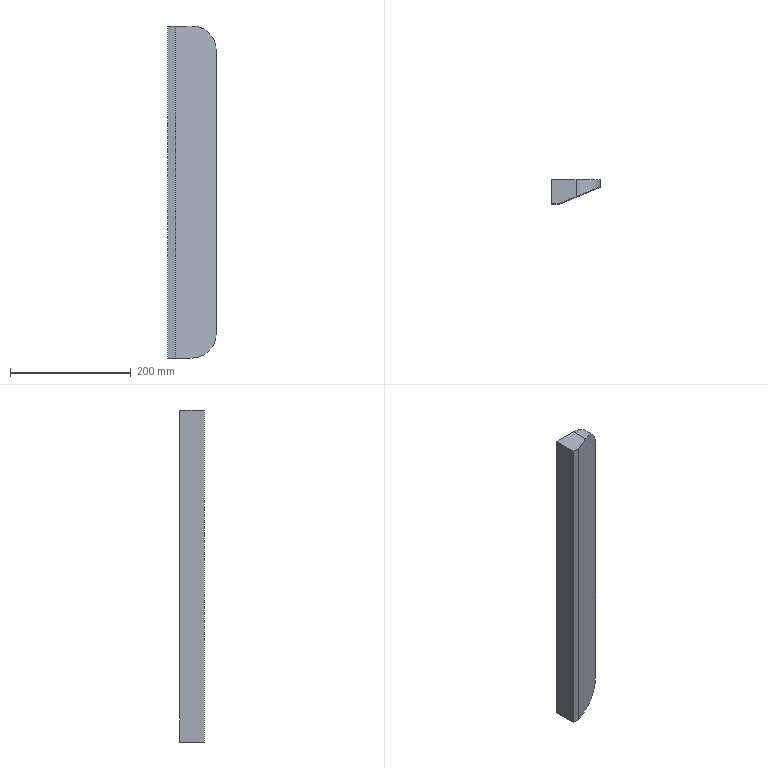Part | SolidWorks | features BaseBody 1 | 1 solid | 9 faces | box 80 x 40 x 550 mm | volume 1225633 mm3 | plane 7 | cylinder 2 | commonest cylinder face diameters 80 x2
STEP:
#1=CARTESIAN_POINT('',(80.,28.,235.));
#2=VERTEX_POINT('',#1);
#3=CARTESIAN_POINT('',(40.,11.529,275.));
#4=VERTEX_POINT('',#3);
#5=CARTESIAN_POINT('',(80.,28.,235.));
#6=CARTESIAN_POINT('',(80.,28.,258.431));
#7=CARTESIAN_POINT('',(63.431,21.178,275.));
#8=CARTESIAN_POINT('',(40.,11.529,275.));
#9=(BOUNDED_CURVE()B_SPLINE_CURVE(3,(#5,#6,#7,#8),.UNSPECIFIED.,.F.,.F.)B_SPLINE_CURVE_WITH_KNOTS((4,4),(0.,1.571),.UNSPECIFIED.)CURVE()GEOMETRIC_REPRESENTATION_ITEM()RATIONAL_B_SPLINE_CURVE((1.,0.8047,0.8047,1.))REPRESENTATION_ITEM(''));
#10=EDGE_CURVE('',#2,#4,#9,.T.);
#11=ORIENTED_EDGE('',*,*,#10,.F.);
#12=CARTESIAN_POINT('',(80.,40.,235.));
#13=VERTEX_POINT('',#12);
#14=CARTESIAN_POINT('',(80.,40.,235.));
#15=DIRECTION('',(0.,-1.,0.));
#16=VECTOR('',#15,1000.);
#17=LINE('',#14,#16);
#18=EDGE_CURVE('',#13,#2,#17,.T.);
#19=ORIENTED_EDGE('',*,*,#18,.F.);
#20=CARTESIAN_POINT('',(40.,40.,275.));
#21=VERTEX_POINT('',#20);
#22=CARTESIAN_POINT('',(40.,40.,235.));
#23=DIRECTION('',(0.,1.,0.));
#24=DIRECTION('',(0.,0.,-1.));
#25=AXIS2_PLACEMENT_3D('',#22,#23,#24);
#26=CIRCLE('',#25,40.);
#27=EDGE_CURVE('',#21,#13,#26,.T.);
#28=ORIENTED_EDGE('',*,*,#27,.F.);
#29=CARTESIAN_POINT('',(40.,0.,275.));
#30=DIRECTION('',(0.,1.,0.));
#31=VECTOR('',#30,1000.);
#32=LINE('',#29,#31);
#33=EDGE_CURVE('',#4,#21,#32,.T.);
#34=ORIENTED_EDGE('',*,*,#33,.F.);
#35=EDGE_LOOP('',(#11,#19,#28,#34));
#36=FACE_OUTER_BOUND('',#35,.T.);
#37=CARTESIAN_POINT('',(40.,0.,235.));
#38=DIRECTION('',(0.,1.,0.));
#39=DIRECTION('',(0.,0.,1.));
#40=AXIS2_PLACEMENT_3D('',#37,#38,#39);
#41=CYLINDRICAL_SURFACE('',#40,40.);
#42=ADVANCED_FACE('',(#36),#41,.T.);
#43=CARTESIAN_POINT('',(40.,11.529,-275.));
#44=VERTEX_POINT('',#43);
#45=CARTESIAN_POINT('',(80.,28.,-235.));
#46=VERTEX_POINT('',#45);
#47=CARTESIAN_POINT('',(40.,11.529,-275.));
#48=CARTESIAN_POINT('',(63.431,21.178,-275.));
#49=CARTESIAN_POINT('',(80.,28.,-258.431));
#50=CARTESIAN_POINT('',(80.,28.,-235.));
#51=(BOUNDED_CURVE()B_SPLINE_CURVE(3,(#47,#48,#49,#50),.UNSPECIFIED.,.F.,.F.)B_SPLINE_CURVE_WITH_KNOTS((4,4),(1.571,3.142),.UNSPECIFIED.)CURVE()GEOMETRIC_REPRESENTATION_ITEM()RATIONAL_B_SPLINE_CURVE((1.,0.8047,0.8047,1.))REPRESENTATION_ITEM(''));
#52=EDGE_CURVE('',#44,#46,#51,.T.);
#53=ORIENTED_EDGE('',*,*,#52,.F.);
#54=CARTESIAN_POINT('',(40.,40.,-275.));
#55=VERTEX_POINT('',#54);
#56=CARTESIAN_POINT('',(40.,28.,-275.));
#57=DIRECTION('',(0.,-1.,0.));
#58=VECTOR('',#57,1000.);
#59=LINE('',#56,#58);
#60=EDGE_CURVE('',#55,#44,#59,.T.);
#61=ORIENTED_EDGE('',*,*,#60,.F.);
#62=CARTESIAN_POINT('',(80.,40.,-235.));
#63=VERTEX_POINT('',#62);
#64=CARTESIAN_POINT('',(40.,40.,-235.));
#65=DIRECTION('',(0.,1.,0.));
#66=DIRECTION('',(0.,0.,-1.));
#67=AXIS2_PLACEMENT_3D('',#64,#65,#66);
#68=CIRCLE('',#67,40.);
#69=EDGE_CURVE('',#63,#55,#68,.T.);
#70=ORIENTED_EDGE('',*,*,#69,.F.);
#71=CARTESIAN_POINT('',(80.,40.,-235.));
#72=DIRECTION('',(0.,1.,0.));
#73=VECTOR('',#72,1000.);
#74=LINE('',#71,#73);
#75=EDGE_CURVE('',#46,#63,#74,.T.);
#76=ORIENTED_EDGE('',*,*,#75,.F.);
#77=EDGE_LOOP('',(#53,#61,#70,#76));
#78=FACE_OUTER_BOUND('',#77,.T.);
#79=CARTESIAN_POINT('',(40.,40.,-235.));
#80=DIRECTION('',(0.,-1.,0.));
#81=DIRECTION('',(0.,0.,-1.));
#82=AXIS2_PLACEMENT_3D('',#79,#80,#81);
#83=CYLINDRICAL_SURFACE('',#82,40.);
#84=ADVANCED_FACE('',(#78),#83,.T.);
#85=CARTESIAN_POINT('',(0.,40.,-275.));
#86=VERTEX_POINT('',#85);
#87=CARTESIAN_POINT('',(0.,40.,-275.));
#88=DIRECTION('',(-1.,0.,0.));
#89=VECTOR('',#88,1000.);
#90=LINE('',#87,#89);
#91=EDGE_CURVE('',#55,#86,#90,.T.);
#92=ORIENTED_EDGE('',*,*,#91,.F.);
#93=ORIENTED_EDGE('',*,*,#60,.T.);
#94=CARTESIAN_POINT('',(12.,0.,-275.));
#95=VERTEX_POINT('',#94);
#96=CARTESIAN_POINT('',(80.,28.,-275.));
#97=DIRECTION('',(0.9247,0.3807,0.));
#98=VECTOR('',#97,1000.);
#99=LINE('',#96,#98);
#100=EDGE_CURVE('',#95,#44,#99,.T.);
#101=ORIENTED_EDGE('',*,*,#100,.F.);
#102=CARTESIAN_POINT('',(0.,0.,-275.));
#103=VERTEX_POINT('',#102);
#104=CARTESIAN_POINT('',(12.,0.,-275.));
#105=DIRECTION('',(1.,0.,0.));
#106=VECTOR('',#105,1000.);
#107=LINE('',#104,#106);
#108=EDGE_CURVE('',#103,#95,#107,.T.);
#109=ORIENTED_EDGE('',*,*,#108,.F.);
#110=CARTESIAN_POINT('',(0.,0.,-275.));
#111=DIRECTION('',(0.,-1.,0.));
#112=VECTOR('',#111,1000.);
#113=LINE('',#110,#112);
#114=EDGE_CURVE('',#86,#103,#113,.T.);
#115=ORIENTED_EDGE('',*,*,#114,.F.);
#116=EDGE_LOOP('',(#92,#93,#101,#109,#115));
#117=FACE_OUTER_BOUND('',#116,.T.);
#118=CARTESIAN_POINT('',(0.,0.,-275.));
#119=DIRECTION('',(0.,0.,-1.));
#120=DIRECTION('',(0.,-1.,0.));
#121=AXIS2_PLACEMENT_3D('',#118,#119,#120);
#122=PLANE('',#121);
#123=ADVANCED_FACE('',(#117),#122,.T.);
#124=CARTESIAN_POINT('',(12.,0.,275.));
#125=VERTEX_POINT('',#124);
#126=CARTESIAN_POINT('',(80.,28.,275.));
#127=DIRECTION('',(0.9247,0.3807,0.));
#128=VECTOR('',#127,1000.);
#129=LINE('',#126,#128);
#130=EDGE_CURVE('',#125,#4,#129,.T.);
#131=ORIENTED_EDGE('',*,*,#130,.T.);
#132=ORIENTED_EDGE('',*,*,#33,.T.);
#133=CARTESIAN_POINT('',(0.,40.,275.));
#134=VERTEX_POINT('',#133);
#135=CARTESIAN_POINT('',(0.,40.,275.));
#136=DIRECTION('',(-1.,0.,0.));
#137=VECTOR('',#136,1000.);
#138=LINE('',#135,#137);
#139=EDGE_CURVE('',#21,#134,#138,.T.);
#140=ORIENTED_EDGE('',*,*,#139,.T.);
#141=CARTESIAN_POINT('',(0.,0.,275.));
#142=VERTEX_POINT('',#141);
#143=CARTESIAN_POINT('',(0.,0.,275.));
#144=DIRECTION('',(0.,-1.,0.));
#145=VECTOR('',#144,1000.);
#146=LINE('',#143,#145);
#147=EDGE_CURVE('',#134,#142,#146,.T.);
#148=ORIENTED_EDGE('',*,*,#147,.T.);
#149=CARTESIAN_POINT('',(12.,0.,275.));
#150=DIRECTION('',(1.,0.,0.));
#151=VECTOR('',#150,1000.);
#152=LINE('',#149,#151);
#153=EDGE_CURVE('',#142,#125,#152,.T.);
#154=ORIENTED_EDGE('',*,*,#153,.T.);
#155=EDGE_LOOP('',(#131,#132,#140,#148,#154));
#156=FACE_OUTER_BOUND('',#155,.T.);
#157=CARTESIAN_POINT('',(0.,0.,275.));
#158=DIRECTION('',(0.,0.,-1.));
#159=DIRECTION('',(0.,-1.,0.));
#160=AXIS2_PLACEMENT_3D('',#157,#158,#159);
#161=PLANE('',#160);
#162=ADVANCED_FACE('',(#156),#161,.F.);
#163=ORIENTED_EDGE('',*,*,#114,.T.);
#164=CARTESIAN_POINT('',(0.,0.,275.));
#165=DIRECTION('',(0.,0.,-1.));
#166=VECTOR('',#165,1000.);
#167=LINE('',#164,#166);
#168=EDGE_CURVE('',#142,#103,#167,.T.);
#169=ORIENTED_EDGE('',*,*,#168,.F.);
#170=ORIENTED_EDGE('',*,*,#147,.F.);
#171=CARTESIAN_POINT('',(0.,40.,275.));
#172=DIRECTION('',(0.,0.,-1.));
#173=VECTOR('',#172,1000.);
#174=LINE('',#171,#173);
#175=EDGE_CURVE('',#134,#86,#174,.T.);
#176=ORIENTED_EDGE('',*,*,#175,.T.);
#177=EDGE_LOOP('',(#163,#169,#170,#176));
#178=FACE_OUTER_BOUND('',#177,.T.);
#179=CARTESIAN_POINT('',(0.,0.,275.));
#180=DIRECTION('',(1.,0.,0.));
#181=DIRECTION('',(0.,1.,0.));
#182=AXIS2_PLACEMENT_3D('',#179,#180,#181);
#183=PLANE('',#182);
#184=ADVANCED_FACE('',(#178),#183,.F.);
#185=CARTESIAN_POINT('',(80.,40.,275.));
#186=DIRECTION('',(0.,0.,-1.));
#187=VECTOR('',#186,1000.);
#188=LINE('',#185,#187);
#189=EDGE_CURVE('',#13,#63,#188,.T.);
#190=ORIENTED_EDGE('',*,*,#189,.T.);
#191=ORIENTED_EDGE('',*,*,#69,.T.);
#192=ORIENTED_EDGE('',*,*,#91,.T.);
#193=ORIENTED_EDGE('',*,*,#175,.F.);
#194=ORIENTED_EDGE('',*,*,#139,.F.);
#195=ORIENTED_EDGE('',*,*,#27,.T.);
#196=EDGE_LOOP('',(#190,#191,#192,#193,#194,#195));
#197=FACE_OUTER_BOUND('',#196,.T.);
#198=CARTESIAN_POINT('',(0.,40.,275.));
#199=DIRECTION('',(0.,-1.,0.));
#200=DIRECTION('',(0.,0.,-1.));
#201=AXIS2_PLACEMENT_3D('',#198,#199,#200);
#202=PLANE('',#201);
#203=ADVANCED_FACE('',(#197),#202,.F.);
#204=CARTESIAN_POINT('',(80.,28.,275.));
#205=DIRECTION('',(0.,0.,-1.));
#206=VECTOR('',#205,1000.);
#207=LINE('',#204,#206);
#208=EDGE_CURVE('',#2,#46,#207,.T.);
#209=ORIENTED_EDGE('',*,*,#208,.T.);
#210=ORIENTED_EDGE('',*,*,#75,.T.);
#211=ORIENTED_EDGE('',*,*,#189,.F.);
#212=ORIENTED_EDGE('',*,*,#18,.T.);
#213=EDGE_LOOP('',(#209,#210,#211,#212));
#214=FACE_OUTER_BOUND('',#213,.T.);
#215=CARTESIAN_POINT('',(80.,40.,275.));
#216=DIRECTION('',(-1.,0.,0.));
#217=DIRECTION('',(0.,0.,1.));
#218=AXIS2_PLACEMENT_3D('',#215,#216,#217);
#219=PLANE('',#218);
#220=ADVANCED_FACE('',(#214),#219,.F.);
#221=ORIENTED_EDGE('',*,*,#100,.T.);
#222=ORIENTED_EDGE('',*,*,#52,.T.);
#223=ORIENTED_EDGE('',*,*,#208,.F.);
#224=ORIENTED_EDGE('',*,*,#10,.T.);
#225=ORIENTED_EDGE('',*,*,#130,.F.);
#226=CARTESIAN_POINT('',(12.,0.,275.));
#227=DIRECTION('',(0.,0.,-1.));
#228=VECTOR('',#227,1000.);
#229=LINE('',#226,#228);
#230=EDGE_CURVE('',#125,#95,#229,.T.);
#231=ORIENTED_EDGE('',*,*,#230,.T.);
#232=EDGE_LOOP('',(#221,#222,#223,#224,#225,#231));
#233=FACE_OUTER_BOUND('',#232,.T.);
#234=CARTESIAN_POINT('',(80.,28.,275.));
#235=DIRECTION('',(-0.3807,0.9247,0.));
#236=DIRECTION('',(0.,0.,1.));
#237=AXIS2_PLACEMENT_3D('',#234,#235,#236);
#238=PLANE('',#237);
#239=ADVANCED_FACE('',(#233),#238,.F.);
#240=ORIENTED_EDGE('',*,*,#108,.T.);
#241=ORIENTED_EDGE('',*,*,#230,.F.);
#242=ORIENTED_EDGE('',*,*,#153,.F.);
#243=ORIENTED_EDGE('',*,*,#168,.T.);
#244=EDGE_LOOP('',(#240,#241,#242,#243));
#245=FACE_OUTER_BOUND('',#244,.T.);
#246=CARTESIAN_POINT('',(12.,0.,275.));
#247=DIRECTION('',(0.,1.,0.));
#248=DIRECTION('',(1.,0.,0.));
#249=AXIS2_PLACEMENT_3D('',#246,#247,#248);
#250=PLANE('',#249);
#251=ADVANCED_FACE('',(#245),#250,.F.);
#252=CLOSED_SHELL('',(#42,#84,#123,#162,#184,#203,#220,#239,#251));
#253=MANIFOLD_SOLID_BREP('',#252);
#254=CARTESIAN_POINT('',(0.,0.,0.));
#255=DIRECTION('',(0.,0.,1.));
#256=DIRECTION('',(1.,0.,0.));
#257=AXIS2_PLACEMENT_3D('',#254,#255,#256);
#258=(LENGTH_UNIT()NAMED_UNIT(*)SI_UNIT(.MILLI.,.METRE.));
#259=UNCERTAINTY_MEASURE_WITH_UNIT(LENGTH_MEASURE(0.00001),#258,'','');
#260=(NAMED_UNIT(*)PLANE_ANGLE_UNIT()SI_UNIT($,.RADIAN.));
#261=(NAMED_UNIT(*)SI_UNIT($,.STERADIAN.)SOLID_ANGLE_UNIT());
#262=(GEOMETRIC_REPRESENTATION_CONTEXT(3)GLOBAL_UNCERTAINTY_ASSIGNED_CONTEXT((#259))GLOBAL_UNIT_ASSIGNED_CONTEXT((#258,#260,#261))REPRESENTATION_CONTEXT('',''));
#263=ADVANCED_BREP_SHAPE_REPRESENTATION('',(#253,#257),#262);